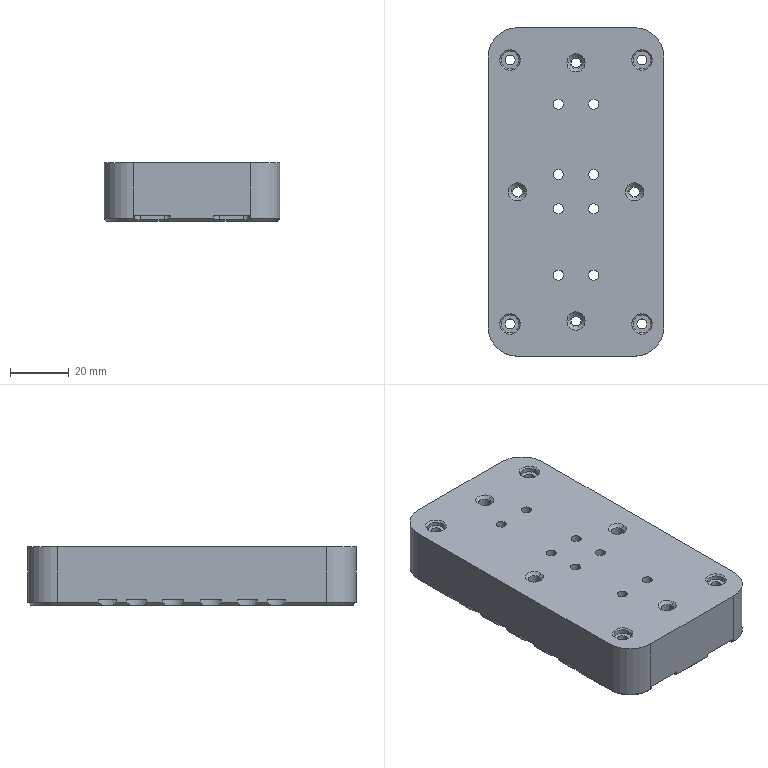Part | SolidWorks | features Cut 6, HoleWzd 6, Chamfer 4, Extrusion 1, Fillet 1, MoveCopyBody 1 | 1 solid | 316 faces | box 60 x 112 x 20 mm | volume 122613 mm3 | cylinder 134 | cone 92 | plane 90 | commonest cylinder face diameters 9 x42 6 x32 3.4 x24 3.3 x8 4 x8 4.2 x8